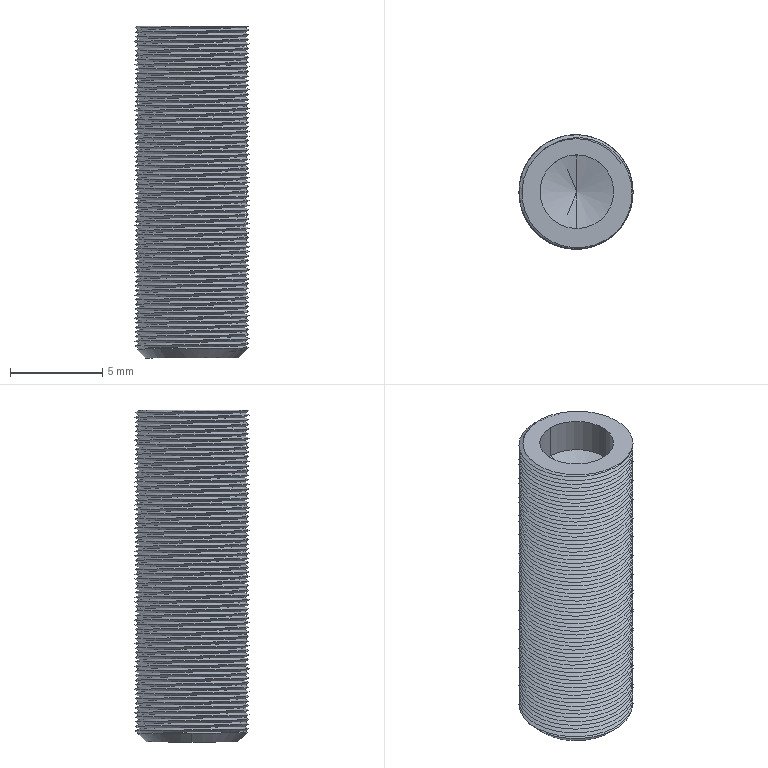Part | SolidWorks | features RefAxis 1 | 1 solid | 24 faces | box 6.183 x 6.183 x 18 mm | volume 451.29 mm3 | plane 9 | cylinder 8 | cone 5 | spline 2 | commonest cylinder face diameters 0.4 x6 4 x2